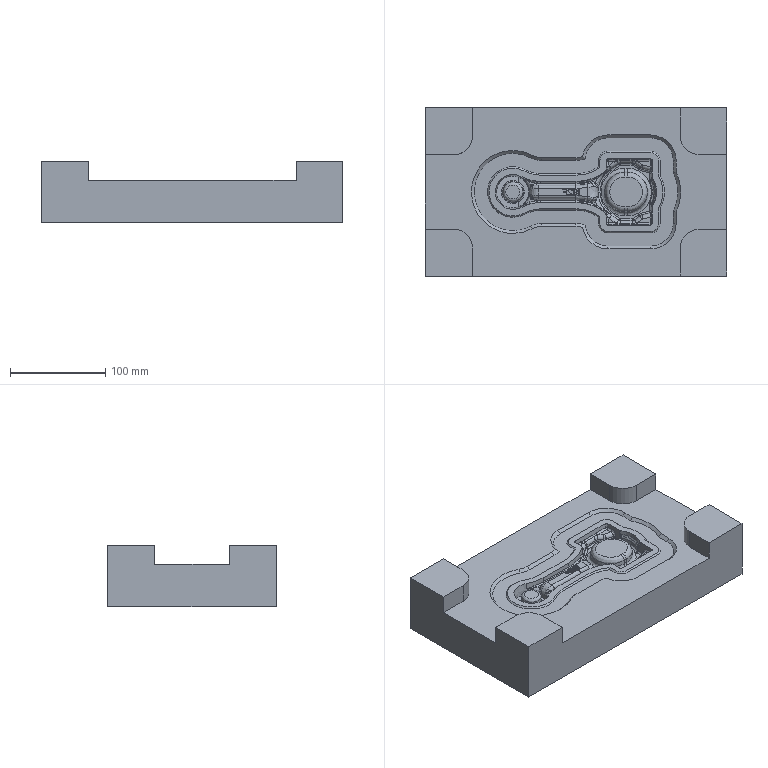NC program | NX | posted with a generic post | part box 317 x 177 x 65 mm
Lines 1 to 1270 of 8842:
N10 G17 G21 G94 G90
(CAVITY_MILL , TOOL : D30R5)
N12 T00 M6
N14 G54
N16 G17 G0 G90 X0.376 Y103.5 S3000 M3
N18 G43 Z10. H0
N20 Z-0.385
N22 G94 G1 Z-0.585 F2500.
N24 Y9.335
N26 X-29.895
N28 G2 X-35.152 Y0. R110.853
N30 X-29.895 Y-9.335 R110.853
N32 G1 X30.647
N34 G2 X35.968 Y0. R110.853
N36 X30.647 Y9.335 R110.854
N38 G1 X0.376
N40 Y22.335
N42 X-38.275
N44 G2 X-50.934 Y0. R97.854
N46 X-38.275 Y-22.335 R97.854
N48 G1 X38.979
N50 G2 X51.814 Y0. R97.854
N52 X38.979 Y22.335 R97.854
N54 G1 X0.376
N56 Y35.335
N58 X-47.513
N60 G2 X-68.015 Y0. R84.854
N62 X-47.513 Y-35.335 R84.854
N64 G1 X48.16
N66 G2 X69.003 Y0. R84.854
N68 X48.16 Y35.335 R84.854
N70 G1 X0.376
N72 Y48.335
N74 X-57.942
N76 G2 X-87.989 Y0. R71.854
N78 X-57.942 Y-48.335 R71.854
N80 G1 X58.519
N82 G2 X89.218 Y0. R71.854
N84 X58.519 Y48.335 R71.854
N86 G1 X0.376
N88 Y61.335
N90 X-70.146
N92 Y58.997
N94 G2 X-129.032 Y0.146 R58.854
N96 G1 X-131.333
N98 Y-0.146
N100 X-128.997
N102 G2 X-70.146 Y-59.052 R58.854
N104 G1 Y-61.335
N106 X70.646
N108 Y-59.5
N110 G2 X129.5 Y-0.646 R58.854
N112 G1 X131.333
N114 Y0.646
N116 X129.5
N118 G2 X70.646 Y59.5 R58.854
N120 G1 Y61.335
N122 X0.376
N124 Y74.335
N126 X-83.146
N128 Y58.997
N130 G2 X-129.029 Y13.146 R45.854
N132 G1 X-144.333
N134 Y-13.146
N136 X-128.998
N138 G2 X-83.146 Y-59.046 R45.854
N140 G1 Y-74.335
N142 X83.646
N144 Y-59.5
N146 G2 X129.5 Y-13.646 R45.854
N148 G1 X144.333
N150 Y13.646
N152 X129.5
N154 G2 X83.646 Y59.5 R45.854
N156 G1 Y74.335
N158 X0.376
N160 Y87.335
N162 X-93.546
N164 Y88.456
N166 X-93.547 Y88.5
N168 X-96.147
N170 X-96.146 Y88.465
N172 Y58.998
N174 G2 X-128.965 Y26.147 R32.854
N176 G1 X-129.03 Y26.146
N178 X-158.453
N180 X-158.5 Y26.147
N182 Y23.547
N184 X-158.451 Y23.546
N186 X-157.333
N188 Y-23.546
N190 X-158.453
N192 X-158.5 Y-23.547
N194 Y-26.147
N196 X-158.453 Y-26.146
N198 X-128.998
N200 G2 X-96.147 Y-58.97 R32.854
N202 G1 X-96.146 Y-59.047
N204 Y-88.456
N206 X-96.147 Y-88.5
N208 X-93.547
N210 X-93.546 Y-88.455
N212 Y-87.335
N214 X94.046
N216 Y-88.456
N218 X94.047 Y-88.5
N220 X96.647
N222 X96.646 Y-88.456
N224 Y-59.5
N226 G2 X129.5 Y-26.646 R32.854
N228 G1 X158.453
N230 X158.5 Y-26.647
N232 Y-24.047
N234 X158.451 Y-24.046
N236 X157.333
N238 Y24.046
N240 X158.453
N242 X158.5 Y24.047
N244 Y26.647
N246 X158.453 Y26.646
N248 X129.5
N250 G2 X96.646 Y59.5 R32.854
N252 G1 Y88.46
N254 X96.647 Y88.5
N256 X94.047
N258 X94.046 Y88.461
N260 Y87.335
N262 X0.376
N264 Y103.5
N266 Z-0.385
N268 G0 Z0.3
N270 X0.372
N272 Z-0.971
N274 G1 Z-1.171
N276 Y10.208
N278 X-28.555
N280 G2 X-34.191 Y0. R111.668
N282 X-31.34 Y-4.849 R111.668
N284 G1 X-22.59 Y-0.009
N286 X-22.479 Y-0.208
N288 X23.257
N290 X23.373 Y0.
N292 X23.257 Y0.208
N294 X-22.479
N296 X-22.594 Y0.
N298 X-22.59 Y-0.009
N300 X-31.34 Y-4.849
N302 G2 X-28.555 Y-10.208 R111.668
N304 G1 X29.3
N306 G2 X35.004 Y0. R111.668
N308 X29.3 Y10.208 R111.668
N310 G1 X0.372
N312 Y23.208
N314 X-37.052
N316 G2 X-49.915 Y0. R98.668
N318 X-37.052 Y-23.208 R98.668
N320 G1 X37.749
N322 G2 X50.79 Y0. R98.668
N324 X37.749 Y23.208 R98.668
N326 G1 X0.372
N328 Y36.208
N330 X-46.419
N332 G2 X-66.887 Y0. R85.668
N334 X-46.419 Y-36.208 R85.668
N336 G1 X47.059
N338 G2 X67.865 Y0. R85.668
N340 X47.059 Y36.208 R85.668
N342 G1 X0.372
N344 Y49.208
N346 X-56.994
N348 G2 X-86.577 Y0. R72.668
N350 X-56.994 Y-49.208 R72.668
N352 G1 X57.564
N354 G2 X87.781 Y0. R72.668
N356 X57.564 Y49.208 R72.668
N358 G1 X0.372
N360 Y62.208
N362 X-69.332
N364 Y59.
N366 G2 X-120.094 Y0. R59.668
N368 G1 X-132.603
N370 X-120.094
N372 G2 X-69.332 Y-59. R59.668
N374 G1 Y-62.208
N376 X69.832
N378 Y-59.492
N380 G2 X125.021 Y0. R59.668
N382 G1 X135.022
N384 X125.021
N386 G2 X69.832 Y59.452 R59.668
N388 G1 Y62.208
N390 X0.372
N392 Y75.208
N394 X-82.332
N396 Y59.
N398 G2 X-129. Y12.332 R46.668
N400 G1 X-145.205
N402 Y-12.332
N404 X-129.
N406 G2 X-82.332 Y-59. R46.668
N408 G1 Y-75.208
N410 X82.832
N412 Y-59.494
N414 G2 X129.533 Y-12.832 R46.668
N416 G1 X145.205
N418 Y12.832
N420 X129.492
N422 G2 X82.832 Y59.458 R46.668
N424 G1 Y75.208
N426 X0.372
N428 Y88.208
N430 X-92.732
N432 Y88.456
N434 Y88.5
N436 X-95.332
N438 Y88.465
N440 Y59.
N442 G2 X-129. Y25.332 R33.668
N444 G1 X-158.453
N446 X-158.5
N448 Y22.732
N450 X-158.451
N452 X-158.205
N454 Y-22.732
N456 X-158.453
N458 X-158.5
N460 Y-25.332
N462 X-158.453
N464 X-129.
N466 G2 X-95.332 Y-59. R33.668
N468 G1 Y-88.456
N470 Y-88.5
N472 X-92.732
N474 Y-88.455
N476 Y-88.208
N478 X93.232
N480 Y-88.456
N482 Y-88.5
N484 X95.832
N486 Y-88.456
N488 Y-59.538
N490 Y-59.496
N492 G2 X129.468 Y-25.832 R33.668
N494 G1 X129.534
N496 X158.453
N498 X158.5
N500 Y-23.232
N502 X158.451
N504 X158.205
N506 Y23.232
N508 X158.453
N510 X158.5
N512 Y25.832
N514 X158.453
N516 X129.534
N518 X129.494
N520 G2 X95.832 Y59.469 R33.668
N522 G1 Y59.538
N524 Y88.46
N526 Y88.5
N528 X93.232
N530 Y88.461
N532 Y88.208
N534 X0.372
N536 Y103.5
N538 Z-0.971
N540 G0 Z-0.285
N542 X0.371
N544 Z-1.556
N546 G1 Z-1.756
N548 Y10.5
N550 X-27.785
N552 G2 X-33.524 Y0. R112.235
N554 X-27.785 Y-10.5 R112.235
N556 G1 X28.526
N558 G2 X34.334 Y0. R112.235
N560 X28.526 Y10.5 R112.235
N562 G1 X22.447
N564 Y0.5
N566 X-21.673
N568 G2 X-21.947 Y0. R122.235
N570 X-21.673 Y-0.5 R122.235
N572 G1 X22.447
N574 G2 X22.724 Y0. R122.235
N576 X22.447 Y0.5 R122.235
N578 G1 Y10.5
N580 X0.371
N582 Y23.5
N584 X-36.332
N586 G2 X-49.209 Y0. R99.235
N588 X-36.332 Y-23.5 R99.235
N590 G1 X37.025
N592 G2 X50.081 Y0. R99.235
N594 X37.025 Y23.5 R99.235
N596 G1 X0.371
N598 Y36.5
N600 X-45.752
N602 G2 X-66.107 Y0. R86.235
N604 X-45.752 Y-36.5 R86.235
N606 G1 X46.389
N608 G2 X67.08 Y0. R86.235
N610 X46.389 Y36.5 R86.235
N612 G1 X0.371
N614 Y49.5
N616 X-56.384
N618 G2 X-85.613 Y0. R73.235
N620 X-56.384 Y-49.5 R73.235
N622 G1 X56.951
N624 G2 X86.802 Y0. R73.235
N626 X56.951 Y49.5 R73.235
N628 G1 X0.371
N630 Y62.5
N632 X-68.765
N634 Y59.
N636 G2 X-116.864 Y0. R60.235
N638 G1 X-131.147
N640 X-116.864
N642 G2 X-68.765 Y-59. R60.235
N644 G1 Y-62.5
N646 X69.265
N648 Y-59.5
N650 G2 X120.118 Y0. R60.235
N652 G1 X132.765
N654 X120.118
N656 G2 X69.265 Y59.5 R60.235
N658 G1 Y62.5
N660 X0.371
N662 Y75.5
N664 X-81.765
N666 Y59.
N668 G2 X-129. Y11.765 R47.235
N670 G1 X-145.5
N672 Y-11.765
N674 X-129.
N676 G2 X-81.765 Y-59. R47.235
N678 G1 Y-75.5
N680 X82.265
N682 Y-59.5
N684 G2 X129.5 Y-12.265 R47.235
N686 G1 X145.5
N688 Y12.265
N690 X129.5
N692 G2 X82.265 Y59.5 R47.235
N694 G1 Y75.5
N696 X0.371
N698 Y88.5
N700 X-94.765
N702 Y88.456
N704 Y59.
N706 G2 X-129. Y24.765 R34.235
N708 G1 X-158.453
N710 X-158.5
N712 Y-24.765
N714 X-158.453
N716 X-129.
N718 G2 X-94.765 Y-59. R34.235
N720 G1 Y-88.456
N722 Y-88.5
N724 X95.265
N726 Y-88.489
N728 Y-59.5
N730 G2 X129.5 Y-25.265 R34.235
N732 G1 X158.453
N734 X158.5
N736 Y25.265
N738 X158.453
N740 X129.5
N742 G2 X95.265 Y59.5 R34.235
N744 G1 Y88.489
N746 Y88.5
N748 X0.371
N750 Y103.5
N752 Z-1.556
N754 G0 Z-0.871
N756 X0.37 Z-2.141
N758 G1 Z-2.341
N760 Y10.5
N762 X-27.323
N764 G2 X-33.034 Y0. R112.652
N766 X-27.323 Y-10.5 R112.652
N768 G1 X28.063
N770 G2 X33.843 Y0. R112.652
N772 X28.063 Y10.5 R112.652
N774 G1 X21.971
N776 Y0.5
N778 X-21.198
N780 G2 X-21.471 Y0. R122.652
N782 X-21.198 Y-0.5 R122.652
N784 G1 X21.971
N786 G2 X22.247 Y0. R122.652
N788 X21.971 Y0.5 R122.652
N790 G1 Y10.5
N792 X0.37
N794 Y23.5
N796 X-35.886
N798 G2 X-48.691 Y0. R99.652
N800 X-35.886 Y-23.5 R99.652
N802 G1 X36.578
N804 G2 X49.561 Y0. R99.652
N806 X36.578 Y23.5 R99.652
N808 G1 X0.37
N810 Y36.5
N812 X-45.32
N814 G2 X-65.537 Y0. R86.652
N816 X-45.32 Y-36.5 R86.652
N818 G1 X45.956
N820 G2 X66.505 Y0. R86.652
N822 X45.956 Y36.5 R86.652
N824 G1 X0.37
N826 Y49.5
N828 X-55.963
N830 G2 X-84.913 Y0. R73.652
N832 X-55.963 Y-49.5 R73.652
N834 G1 X56.53
N836 G2 X86.091 Y0. R73.652
N838 X56.53 Y49.5 R73.652
N840 G1 X0.37
N842 Y62.5
N844 X-68.348
N846 Y58.996
N848 G2 X-114.94 Y0. R60.652
N850 G1 X-130.143
N852 X-114.94
N854 G2 X-68.348 Y-59.052 R60.652
N856 G1 Y-62.5
N858 X68.848
N860 Y-59.5
N862 G2 X117.735 Y0. R60.652
N864 G1 X131.583
N866 X117.735
N868 G2 X68.848 Y59.5 R60.652
N870 G1 Y62.5
N872 X0.37
N874 Y75.5
N876 X-81.348
N878 Y58.997
N880 G2 X-129.029 Y11.348 R47.652
N882 G1 X-145.5
N884 Y-11.348
N886 X-128.998
N888 G2 X-81.348 Y-59.046 R47.652
N890 G1 Y-75.5
N892 X81.848
N894 Y-59.5
N896 G2 X129.5 Y-11.848 R47.652
N898 G1 X145.5
N900 Y11.848
N902 X129.5
N904 G2 X81.848 Y59.5 R47.652
N906 G1 Y75.5
N908 X0.37
N910 Y88.5
N912 X-94.348
N914 Y88.456
N916 Y59.047
N918 Y58.998
N920 G2 X-128.965 Y24.348 R34.652
N922 G1 X-129.03
N924 X-158.453
N926 X-158.5
N928 Y-24.348
N930 X-158.453
N932 X-128.998
N934 G2 X-94.348 Y-58.97 R34.652
N936 G1 Y-59.047
N938 Y-88.456
N940 Y-88.5
N942 X94.848
N944 Y-88.493
N946 Y-59.5
N948 G2 X129.5 Y-24.848 R34.652
N950 G1 X158.453
N952 X158.5
N954 Y24.848
N956 X158.453
N958 X129.5
N960 G2 X94.848 Y59.5 R34.652
N962 G1 Y88.493
N964 Y88.5
N966 X0.37
N968 Y103.5
N970 Z-2.141
N972 G0 Z-1.456
N974 Z-2.726
N976 G1 Z-2.926
N978 Y10.5
N980 X-20.848
N982 Y0.5
N984 G2 X-21.12 Y0. R122.959
N986 X-20.848 Y-0.5 R122.959
N988 G1 X21.62
N990 G2 X21.895 Y0. R122.959
N992 X21.62 Y0.5 R122.959
N994 G1 X-20.848
N996 Y10.5
N998 X-26.982
N1000 G2 X-32.673 Y0. R112.959
N1002 X-26.982 Y-10.5 R112.959
N1004 G1 X27.722
N1006 G2 X33.481 Y0. R112.959
N1008 X27.722 Y10.5 R112.959
N1010 G1 X0.37
N1012 Y23.5
N1014 X-35.557
N1016 G2 X-48.31 Y0. R99.959
N1018 X-35.557 Y-23.5 R99.959
N1020 G1 X36.248
N1022 G2 X49.178 Y0. R99.959
N1024 X36.248 Y23.5 R99.959
N1026 G1 X0.37
N1028 Y36.5
N1030 X-45.002
N1032 G2 X-65.118 Y0. R86.959
N1034 X-45.002 Y-36.5 R86.959
N1036 G1 X45.637
N1038 G2 X66.083 Y0. R86.959
N1040 X45.637 Y36.5 R86.959
N1042 G1 X0.37
N1044 Y49.5
N1046 X-55.653
N1048 G2 X-84.402 Y0. R73.959
N1050 X-55.653 Y-49.5 R73.959
N1052 G1 X56.22
N1054 G2 X85.571 Y0. R73.959
N1056 X56.22 Y49.5 R73.959
N1058 G1 X0.37
N1060 Y62.5
N1062 X-68.041
N1064 Y59.
N1066 G2 X-113.669 Y0. R60.959
N1068 G1 X-129.411
N1070 X-113.669
N1072 G2 X-68.041 Y-59. R60.959
N1074 G1 Y-62.5
N1076 X68.541
N1078 Y-59.5
N1080 G2 X116.241 Y0. R60.959
N1082 G1 X130.82
N1084 X116.241
N1086 G2 X68.541 Y59.5 R60.959
N1088 G1 Y62.5
N1090 X0.37
N1092 Y75.5
N1094 X-81.041
N1096 Y59.
N1098 G2 X-129. Y11.041 R47.959
N1100 G1 X-145.5
N1102 Y-11.041
N1104 X-129.
N1106 G2 X-81.041 Y-59. R47.959
N1108 G1 Y-75.5
N1110 X81.541
N1112 Y-59.5
N1114 G2 X129.5 Y-11.541 R47.959
N1116 G1 X145.5
N1118 Y11.541
N1120 X129.5
N1122 G2 X81.541 Y59.5 R47.959
N1124 G1 Y75.5
N1126 X0.37
N1128 Y88.5
N1130 X-94.041
N1132 Y88.496
N1134 Y59.
N1136 G2 X-129. Y24.041 R34.959
N1138 G1 X-158.496
N1140 X-158.5
N1142 Y-24.041
N1144 X-158.496
N1146 X-129.
N1148 G2 X-94.041 Y-59. R34.959
N1150 G1 Y-88.496
N1152 Y-88.5
N1154 X94.541
N1156 Y-88.496
N1158 Y-59.5
N1160 G2 X129.5 Y-24.541 R34.959
N1162 G1 X158.453
N1164 X158.5
N1166 Y24.541
N1168 X158.453
N1170 X129.5
N1172 G2 X94.541 Y59.5 R34.959
N1174 G1 Y88.496
N1176 Y88.5
N1178 X0.37
N1180 Y103.5
N1182 Z-2.726
N1184 G0 Z-2.041
N1186 X0.369 Z-3.312
N1188 G1 Z-3.512
N1190 Y10.5
N1192 X-20.6
N1194 Y0.5
N1196 G2 X-20.871 Y0. R123.178
N1198 X-20.6 Y-0.5 R123.178
N1200 G1 X21.371
N1202 G2 X21.646 Y0. R123.178
N1204 X21.371 Y0.5 R123.178
N1206 G1 X-20.6
N1208 Y10.5
N1210 X-26.74
N1212 G2 X-32.417 Y0. R113.178
N1214 X-26.74 Y-10.5 R113.178
N1216 G1 X27.479
N1218 G2 X33.224 Y0. R113.178
N1220 X27.479 Y10.5 R113.178
N1222 G1 X0.369
N1224 Y23.5
N1226 X-35.323
N1228 G2 X-48.039 Y0. R100.178
N1230 X-35.323 Y-23.5 R100.178
N1232 G1 X36.014
N1234 G2 X48.906 Y0. R100.178
N1236 X36.014 Y23.5 R100.178
N1238 G1 X0.369
N1240 Y36.5
N1242 X-44.776
N1244 G2 X-64.82 Y0. R87.178
N1246 X-44.776 Y-36.5 R87.178
N1248 G1 X45.411
N1250 G2 X65.784 Y0. R87.178
N1252 X45.411 Y36.5 R87.178
N1254 G1 X0.369
N1256 Y49.5
N1258 X-55.433
N1260 G2 X-84.04 Y0. R74.178
N1262 X-55.433 Y-49.5 R74.178
N1264 G1 X55.999
N1266 G2 X85.204 Y0. R74.178
N1268 X55.999 Y49.5 R74.178
N1270 G1 X0.369
N1272 Y62.5
N1274 X-67.822
N1276 Y59.
N1278 G2 X-112.821 Y0. R61.178
N1280 G1 X-128.854
N1282 X-112.821
N1284 G2 X-67.822 Y-59. R61.178
N1286 G1 Y-62.5
N1288 X68.322
N1290 Y-59.5
N1292 G2 X115.27 Y0. R61.178
N1294 G1 X130.301
N1296 X115.27
N1298 G2 X68.322 Y59.5 R61.178
N1300 G1 Y62.5
N1302 X0.369
N1304 Y75.5
N1306 X-80.822
N1308 Y59.
N1310 G2 X-129. Y10.822 R48.178
N1312 G1 X-145.5
N1314 Y-10.822
N1316 X-129.
N1318 G2 X-80.822 Y-59. R48.178
N1320 G1 Y-75.5
N1322 X81.322
N1324 Y-59.5
N1326 G2 X129.5 Y-11.322 R48.178
N1328 G1 X145.5
N1330 Y11.322
N1332 X129.5
N1334 G2 X81.322 Y59.5 R48.178
N1336 G1 Y75.5
N1338 X0.369
N1340 Y88.5
N1342 X-93.822
N1344 Y88.498
N1346 Y59.
N1348 G2 X-129. Y23.822 R35.178
N1350 G1 X-158.498
N1352 X-158.5
N1354 Y-23.822
N1356 X-158.498
N1358 X-129.
N1360 G2 X-93.822 Y-59. R35.178
N1362 G1 Y-88.498
N1364 Y-88.5
N1366 X94.322
N1368 Y-88.498
N1370 Y-59.5
N1372 G2 X129.5 Y-24.322 R35.178
N1374 G1 X158.453
N1376 X158.5
N1378 Y24.322
N1380 X158.453
N1382 X129.5
N1384 G2 X94.322 Y59.5 R35.178
N1386 G1 Y88.498
N1388 Y88.5
N1390 X0.369
N1392 Y103.5
N1394 Z-3.312
N1396 G0 Z-2.626
N1398 Z-3.897
N1400 G1 Z-4.097
N1402 Y10.5
N1404 X-20.439
N1406 Y0.5
N1408 G2 X-20.71 Y0. R123.319
N1410 X-20.439 Y-0.5 R123.319
N1412 G1 X21.21
N1414 G2 X21.484 Y0. R123.319
N1416 X21.21 Y0.5 R123.319
N1418 G1 X-20.439
N1420 Y10.5
N1422 X-26.584
N1424 G2 X-32.251 Y0. R113.319
N1426 X-26.584 Y-10.5 R113.319
N1428 G1 X27.322
N1430 G2 X33.058 Y0. R113.319
N1432 X27.322 Y10.5 R113.319
N1434 G1 X0.369
N1436 Y23.5
N1438 X-35.172
N1440 G2 X-47.864 Y0. R100.319
N1442 X-35.172 Y-23.5 R100.319
N1444 G1 X35.862
N1446 G2 X48.73 Y0. R100.319
N1448 X35.862 Y23.5 R100.319
N1450 G1 X0.369
N1452 Y36.5
N1454 X-44.629
N1456 G2 X-64.629 Y0. R87.319
N1458 X-44.629 Y-36.5 R87.319
N1460 G1 X45.264
N1462 G2 X65.59 Y0. R87.319
N1464 X45.264 Y36.5 R87.319
N1466 G1 X0.369
N1468 Y49.5
N1470 X-55.29
N1472 G2 X-83.807 Y0. R74.319
N1474 X-55.29 Y-49.5 R74.319
N1476 G1 X55.856
N1478 G2 X84.968 Y0. R74.319
N1480 X55.856 Y49.5 R74.319
N1482 G1 X0.369
N1484 Y62.5
N1486 X-67.681
N1488 Y59.
N1490 G2 X-112.295 Y0. R61.319
N1492 G1 X-128.453
N1494 X-112.295
N1496 G2 X-67.681 Y-59. R61.319
N1498 G1 Y-62.5
N1500 X68.181
N1502 Y-59.5
N1504 G2 X114.674 Y0. R61.319
N1506 G1 X129.966
N1508 X114.674
N1510 G2 X68.181 Y59.5 R61.319
N1512 G1 Y62.5
N1514 X0.369
N1516 Y75.5
N1518 X-80.681
N1520 Y59.
N1522 G2 X-129. Y10.681 R48.319
N1524 G1 X-145.5
N1526 Y-10.681
N1528 X-129.
N1530 G2 X-80.681 Y-59. R48.319
N1532 G1 Y-75.5
N1534 X81.181
N1536 Y-59.5
N1538 G2 X129.5 Y-11.181 R48.319
N1540 G1 X145.5
N1542 Y11.181
N1544 X129.5
N1546 G2 X81.181 Y59.5 R48.319
N1548 G1 Y75.5
N1550 X0.369
N1552 Y88.5
N1554 X-93.681
N1556 Y59.
N1558 G2 X-129. Y23.681 R35.319
N1560 G1 X-158.5
N1562 Y-23.681
N1564 X-129.
N1566 G2 X-93.681 Y-59. R35.319
N1568 G1 Y-88.499
N1570 X94.181 Y-88.5
N1572 Y-59.5
N1574 G2 X129.5 Y-24.181 R35.319
N1576 G1 X158.499
N1578 X158.5 Y24.181
N1580 X129.5
N1582 G2 X94.181 Y59.5 R35.319
N1584 G1 Y88.5
N1586 X0.369
N1588 Y103.5
N1590 Z-3.897
N1592 G0 Z-3.212
N1594 Z-4.482
N1596 G1 Z-4.682
N1598 Y10.5
N1600 X-26.506
N1602 G2 X-29.164 Y5.241 R113.39
N1604 G1 X-20.359 Y0.5
N1606 G2 X-20.63 Y0. R123.39
N1608 X-20.359 Y-0.5 R123.39
N1610 G1 X21.13
N1612 G2 X21.403 Y0. R123.39
N1614 X21.13 Y0.5 R123.39
N1616 G1 X-20.359
N1618 X-29.164 Y5.241
N1620 G2 X-32.169 Y0. R113.39
N1622 X-26.506 Y-10.5 R113.39
N1624 G1 X27.244
N1626 G2 X32.975 Y0. R113.39
N1628 X27.244 Y10.5 R113.39
N1630 G1 X0.369
N1632 Y23.5
N1634 X-35.096
N1636 G2 X-47.777 Y0. R100.39
N1638 X-35.096 Y-23.5 R100.39
N1640 G1 X35.787
N1642 G2 X48.643 Y0. R100.39
N1644 X35.787 Y23.5 R100.39
N1646 G1 X0.369
N1648 Y36.5
N1650 X-44.556
N1652 G2 X-64.533 Y0. R87.39
N1654 X-44.556 Y-36.5 R87.39
N1656 G1 X45.191
N1658 G2 X65.494 Y0. R87.39
N1660 X45.191 Y36.5 R87.39
N1662 G1 X0.369
N1664 Y49.5
N1666 X-55.219
N1668 G2 X-83.691 Y0. R74.39
N1670 X-55.219 Y-49.5 R74.39
N1672 G1 X55.785
N1674 G2 X84.85 Y0. R74.39
N1676 X55.785 Y49.5 R74.39
N1678 G1 X0.369
N1680 Y62.5
N1682 X-67.61
N1684 Y59.
N1686 G2 X-112.037 Y0. R61.39
N1688 G1 X-128.231
N1690 X-112.037
N1692 G2 X-67.61 Y-59. R61.39
N1694 G1 Y-62.5
N1696 X68.11
N1698 Y-59.5
N1700 G2 X114.384 Y0. R61.39
N1702 G1 X129.796
N1704 X114.384
N1706 G2 X68.11 Y59.5 R61.39
N1708 G1 Y62.5
N1710 X0.369
N1712 Y75.5
N1714 X-80.61
N1716 Y59.
N1718 G2 X-129. Y10.61 R48.39
N1720 G1 X-145.5
N1722 Y-10.61
N1724 X-129.
N1726 G2 X-80.61 Y-59. R48.39
N1728 G1 Y-75.5
N1730 X81.11
N1732 Y-59.5
N1734 G2 X129.5 Y-11.11 R48.39
N1736 G1 X145.5
N1738 Y11.11
N1740 X129.5
N1742 G2 X81.11 Y59.5 R48.39
N1744 G1 Y75.5
N1746 X0.369
N1748 Y88.5
N1750 X-93.61
N1752 Y59.
N1754 G2 X-129. Y23.61 R35.39
N1756 G1 X-158.5
N1758 Y-23.61
N1760 X-129.
N1762 G2 X-93.61 Y-59. R35.39
N1764 G1 Y-88.5
N1766 X94.11
N1768 Y-59.5
N1770 G2 X129.5 Y-24.11 R35.39
N1772 G1 X158.5
N1774 Y24.11
N1776 X129.5
N1778 G2 X94.11 Y59.5 R35.39
N1780 G1 Y88.5
N1782 X0.369
N1784 Y103.5
N1786 Z-4.482
N1788 G0 Z-3.797
N1790 Z-5.068
N1792 G1 Z-5.268
N1794 Y10.5
N1796 X-26.495
N1798 G2 X-29.153 Y5.241 R113.4
N1800 G1 X-20.348 Y0.5
N1802 G2 X-20.618 Y0. R123.4
N1804 X-20.348 Y-0.5 R123.4
N1806 G1 X21.118
N1808 G2 X21.392 Y0. R123.4
N1810 X21.118 Y0.5 R123.4
N1812 G1 X-20.348
N1814 X-29.153 Y5.241
N1816 G2 X-32.157 Y0. R113.4
N1818 X-26.495 Y-10.5 R113.4
N1820 G1 X27.233
N1822 G2 X32.963 Y0. R113.4
N1824 X27.233 Y10.5 R113.4
N1826 G1 X0.369
N1828 Y23.5
N1830 X-35.086
N1832 G2 X-47.765 Y0. R100.4
N1834 X-35.086 Y-23.5 R100.4
N1836 G1 X35.776
N1838 G2 X48.63 Y0. R100.4
N1840 X35.776 Y23.5 R100.4
N1842 G1 X0.369
N1844 Y36.5
N1846 X-44.546
N1848 G2 X-64.519 Y0. R87.4
N1850 X-44.546 Y-36.5 R87.4
N1852 G1 X45.181
N1854 G2 X65.48 Y0. R87.4
N1856 X45.181 Y36.5 R87.4
N1858 G1 X0.369
N1860 Y49.5
N1862 X-55.209
N1864 G2 X-83.675 Y0. R74.4
N1866 X-55.209 Y-49.5 R74.4
N1868 G1 X55.775
N1870 G2 X84.833 Y0. R74.4
N1872 X55.775 Y49.5 R74.4
N1874 G1 X0.369
N1876 Y62.5
N1878 X-67.6
N1880 Y59.
N1882 G2 X-112.001 Y0. R61.4
N1884 G1 X-128.198
N1886 X-112.001
N1888 G2 X-67.6 Y-59. R61.4
N1890 G1 Y-62.5
N1892 X68.1
N1894 Y-59.5
N1896 G2 X114.344 Y0. R61.4
N1898 G1 X129.772
N1900 X114.344
N1902 G2 X68.1 Y59.5 R61.4
N1904 G1 Y62.5
N1906 X0.369
N1908 Y75.5
N1910 X-80.6
N1912 Y59.
N1914 G2 X-129. Y10.6 R48.4
N1916 G1 X-145.5
N1918 Y-10.6
N1920 X-129.
N1922 G2 X-80.6 Y-59. R48.4
N1924 G1 Y-75.5
N1926 X81.1
N1928 Y-59.5
N1930 G2 X129.5 Y-11.1 R48.4
N1932 G1 X145.5
N1934 Y11.1
N1936 X129.5
N1938 G2 X81.1 Y59.5 R48.4
N1940 G1 Y75.5
N1942 X0.369
N1944 Y88.5
N1946 X-93.6
N1948 Y59.
N1950 G2 X-129. Y23.6 R35.4
N1952 G1 X-158.5
N1954 Y-23.6
N1956 X-129.
N1958 G2 X-93.6 Y-59. R35.4
N1960 G1 Y-88.5
N1962 X94.1
N1964 Y-59.5
N1966 G2 X129.5 Y-24.1 R35.4
N1968 G1 X158.5
N1970 Y24.1
N1972 X129.5
N1974 G2 X94.1 Y59.5 R35.4
N1976 G1 Y88.5
N1978 X0.369
N1980 Y103.5
N1982 Z-5.068
N1984 G0 Z-4.382
N1986 Z-5.653
N1988 G1 Z-5.853
N1990 Y10.5
N1992 X-26.495
N1994 G2 X-29.153 Y5.241 R113.4
N1996 G1 X-20.348 Y0.5
N1998 G2 X-20.618 Y0. R123.4
N2000 X-20.348 Y-0.5 R123.4
N2002 G1 X21.118
N2004 G2 X21.392 Y0. R123.4
N2006 X21.118 Y0.5 R123.4
N2008 G1 X-20.348
N2010 X-29.153 Y5.241
N2012 G2 X-32.157 Y0. R113.4
N2014 X-26.495 Y-10.5 R113.4
N2016 G1 X27.233
N2018 G2 X32.963 Y0. R113.4
N2020 X27.233 Y10.5 R113.4
N2022 G1 X0.369
N2024 Y23.5
N2026 X-35.086
N2028 G2 X-47.765 Y0. R100.4
N2030 X-35.086 Y-23.5 R100.4
N2032 G1 X35.776
N2034 G2 X48.63 Y0. R100.4
N2036 X35.776 Y23.5 R100.4
N2038 G1 X0.369
N2040 Y36.5
N2042 X-44.546
N2044 G2 X-64.519 Y0. R87.4
N2046 X-44.546 Y-36.5 R87.4
N2048 G1 X45.181
N2050 G2 X65.48 Y0. R87.4
N2052 X45.181 Y36.5 R87.4
N2054 G1 X0.369
N2056 Y49.5
N2058 X-55.209
N2060 G2 X-83.675 Y0. R74.4
N2062 X-55.209 Y-49.5 R74.4
N2064 G1 X55.775
N2066 G2 X84.833 Y0. R74.4
N2068 X55.775 Y49.5 R74.4
N2070 G1 X0.369
N2072 Y62.5
N2074 X-67.6
N2076 Y59.
N2078 G2 X-112.001 Y0. R61.4
N2080 G1 X-128.198
N2082 X-112.001
N2084 G2 X-67.6 Y-59. R61.4
N2086 G1 Y-62.5
N2088 X68.1
N2090 Y-59.5
N2092 G2 X114.344 Y0. R61.4
N2094 G1 X129.772
N2096 X114.344
N2098 G2 X68.1 Y59.5 R61.4
N2100 G1 Y62.5
N2102 X0.369
N2104 Y75.5
N2106 X-80.6
N2108 Y59.
N2110 G2 X-129. Y10.6 R48.4
N2112 G1 X-145.5
N2114 Y-10.6
N2116 X-129.
N2118 G2 X-80.6 Y-59. R48.4
N2120 G1 Y-75.5
N2122 X81.1
N2124 Y-59.5
N2126 G2 X129.5 Y-11.1 R48.4
N2128 G1 X145.5
N2130 Y11.1
N2132 X129.5
N2134 G2 X81.1 Y59.5 R48.4
N2136 G1 Y75.5
N2138 X0.369
N2140 Y88.5
N2142 X-93.6
N2144 Y59.
N2146 G2 X-129. Y23.6 R35.4
N2148 G1 X-158.5
N2150 Y-23.6
N2152 X-129.
N2154 G2 X-93.6 Y-59. R35.4
N2156 G1 Y-88.5
N2158 X94.1
N2160 Y-59.5
N2162 G2 X129.5 Y-24.1 R35.4
N2164 G1 X158.5
N2166 Y24.1
N2168 X129.5
N2170 G2 X94.1 Y59.5 R35.4
N2172 G1 Y88.5
N2174 X0.369
N2176 Y103.5
N2178 Z-5.653
N2180 G0 Z-4.968
N2182 Z-6.238
N2184 G1 Z-6.438
N2186 Y10.5
N2188 X-26.495
N2190 G2 X-32.157 Y0. R113.4
N2192 X-26.495 Y-10.5 R113.4
N2194 G1 X27.233
N2196 G2 X32.963 Y0. R113.4
N2198 X27.233 Y10.5 R113.4
N2200 G1 X21.118
N2202 Y0.5
N2204 X-20.348
N2206 G2 X-20.618 Y0. R123.4
N2208 X-20.348 Y-0.5 R123.4
N2210 G1 X21.118
N2212 G2 X21.392 Y0. R123.4
N2214 X21.118 Y0.5 R123.4
N2216 G1 Y10.5
N2218 X0.369
N2220 Y23.5
N2222 X-35.086
N2224 G2 X-47.765 Y0. R100.4
N2226 X-35.086 Y-23.5 R100.4
N2228 G1 X35.776
N2230 G2 X48.63 Y0. R100.4
N2232 X35.776 Y23.5 R100.4
N2234 G1 X0.369
N2236 Y36.5
N2238 X-44.546
N2240 G2 X-64.519 Y0. R87.4
N2242 X-44.546 Y-36.5 R87.4
N2244 G1 X45.181
N2246 G2 X65.48 Y0. R87.4
N2248 X45.181 Y36.5 R87.4
N2250 G1 X0.369
N2252 Y49.5
N2254 X-55.209
N2256 G2 X-83.675 Y0. R74.4
N2258 X-55.209 Y-49.5 R74.4
N2260 G1 X55.775
N2262 G2 X84.833 Y0. R74.4
N2264 X55.775 Y49.5 R74.4
N2266 G1 X0.369
N2268 Y62.5
N2270 X-67.6
N2272 Y59.
N2274 G2 X-112.001 Y0. R61.4
N2276 G1 X-128.198
N2278 X-112.001
N2280 G2 X-67.6 Y-59. R61.4
N2282 G1 Y-62.5
N2284 X68.1
N2286 Y-59.5
N2288 G2 X114.344 Y0. R61.4
N2290 G1 X129.772
N2292 X114.344
N2294 G2 X68.1 Y59.5 R61.4
N2296 G1 Y62.5
N2298 X0.369
N2300 Y75.5
N2302 X-80.6
N2304 Y59.
N2306 G2 X-129. Y10.6 R48.4
N2308 G1 X-145.5
N2310 Y-10.6
N2312 X-129.
N2314 G2 X-80.6 Y-59. R48.4
N2316 G1 Y-75.5
N2318 X81.1
N2320 Y-59.5
N2322 G2 X129.5 Y-11.1 R48.4
N2324 G1 X145.5
N2326 Y11.1
N2328 X129.5
N2330 G2 X81.1 Y59.5 R48.4
N2332 G1 Y75.5
N2334 X0.369
N2336 Y88.5
N2338 X-93.6
N2340 Y59.
N2342 G2 X-129. Y23.6 R35.4
N2344 G1 X-158.5
N2346 Y-23.6
N2348 X-129.
N2350 G2 X-93.6 Y-59. R35.4
N2352 G1 Y-88.5
N2354 X94.1
N2356 Y-59.5
N2358 G2 X129.5 Y-24.1 R35.4
N2360 G1 X158.5
N2362 Y24.1
N2364 X129.5
N2366 G2 X94.1 Y59.5 R35.4
N2368 G1 Y88.5
N2370 X0.369
N2372 Y103.5
N2374 Z-6.238
N2376 G0 Z-5.553
N2378 Z-6.824
N2380 G1 Z-7.024
N2382 Y10.5
N2384 X-26.495
N2386 G2 X-32.157 Y0. R113.4
N2388 X-26.495 Y-10.5 R113.4
N2390 G1 X27.233
N2392 G2 X32.963 Y0. R113.4
N2394 X27.233 Y10.5 R113.4
N2396 G1 X21.118
N2398 Y0.5
N2400 X-20.348
N2402 G2 X-20.618 Y0. R123.4
N2404 X-20.348 Y-0.5 R123.4
N2406 G1 X21.118
N2408 G2 X21.392 Y0. R123.4
N2410 X21.118 Y0.5 R123.4
N2412 G1 Y10.5
N2414 X0.369
N2416 Y23.5
N2418 X-35.086
N2420 G2 X-47.765 Y0. R100.4
N2422 X-35.086 Y-23.5 R100.4
N2424 G1 X35.776
N2426 G2 X48.63 Y0. R100.4
N2428 X35.776 Y23.5 R100.4
N2430 G1 X0.369
N2432 Y36.5
N2434 X-44.546
N2436 G2 X-64.519 Y0. R87.4
N2438 X-44.546 Y-36.5 R87.4
N2440 G1 X45.181
N2442 G2 X65.48 Y0. R87.4
N2444 X45.181 Y36.5 R87.4
N2446 G1 X0.369
N2448 Y49.5
N2450 X-55.209
N2452 G2 X-83.675 Y0. R74.4
N2454 X-55.209 Y-49.5 R74.4
N2456 G1 X55.775
N2458 G2 X84.833 Y0. R74.4
N2460 X55.775 Y49.5 R74.4
N2462 G1 X0.369
N2464 Y62.5
N2466 X-67.6
N2468 Y59.
N2470 G2 X-112.001 Y0. R61.4
N2472 G1 X-128.198
N2474 X-112.001
N2476 G2 X-67.6 Y-59. R61.4
N2478 G1 Y-62.5
N2480 X68.1
N2482 Y-59.5
N2484 G2 X114.344 Y0. R61.4
N2486 G1 X129.772
N2488 X114.344
N2490 G2 X68.1 Y59.5 R61.4
N2492 G1 Y62.5
N2494 X0.369
N2496 Y75.5
N2498 X-80.6
N2500 Y59.
N2502 G2 X-129. Y10.6 R48.4
N2504 G1 X-145.5
N2506 Y-10.6
N2508 X-129.
N2510 G2 X-80.6 Y-59. R48.4
N2512 G1 Y-75.5
N2514 X81.1
N2516 Y-59.5
N2518 G2 X129.5 Y-11.1 R48.4
N2520 G1 X145.5
N2522 Y11.1
N2524 X129.5
N2526 G2 X81.1 Y59.5 R48.4
N2528 G1 Y75.5
N2530 X0.369
N2532 Y88.5
N2534 X-93.6
N2536 Y59.
N2538 G2 X-129. Y23.6 R35.4